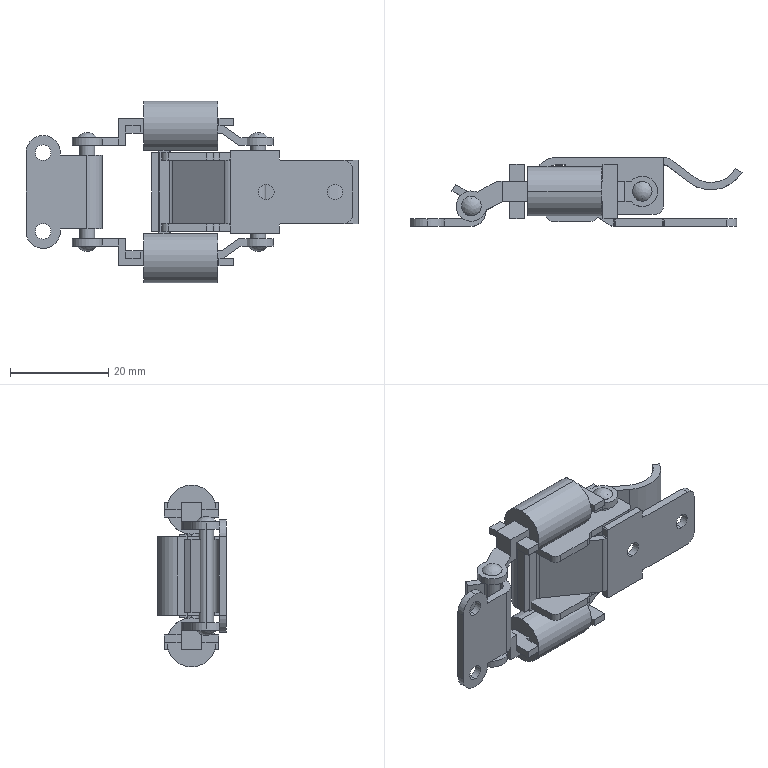Part | SolidWorks | 4 solids | 212 faces | box 67.583 x 14 x 37 mm | volume 6492 mm3 | plane 131 | cylinder 77 | sphere 4 | commonest cylinder face diameters 3 x14 3.2 x14 4 x11 6.2 x10 0.4 x8 10 x4